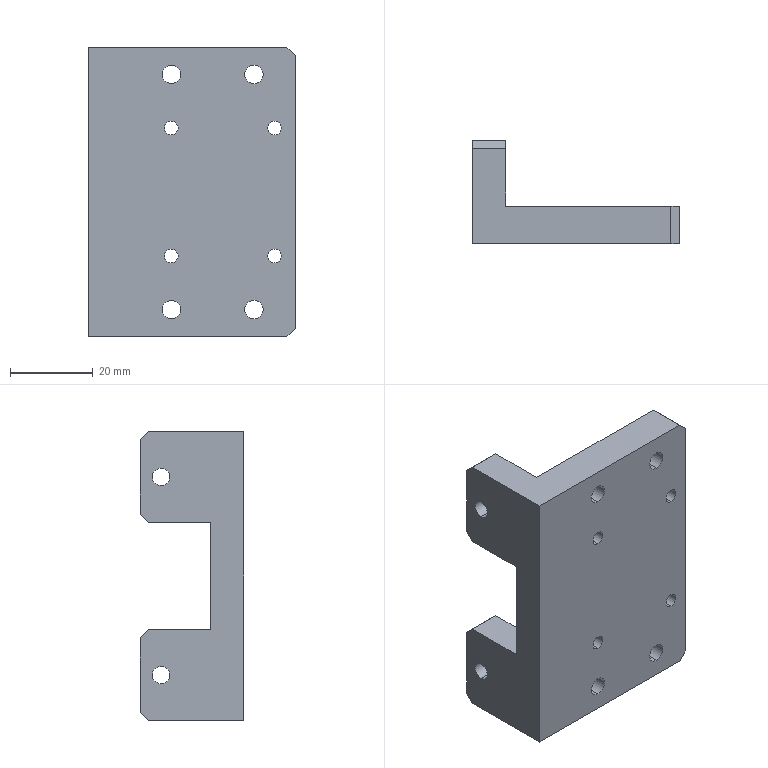Part | SolidWorks | features BaseBody 1 | 1 solid | 52 faces | box 50 x 25 x 70 mm | volume 34025 mm3 | cylinder 28 | plane 24 | commonest cylinder face diameters 3.3 x8 4.5 x8 8 x8 4.2 x4